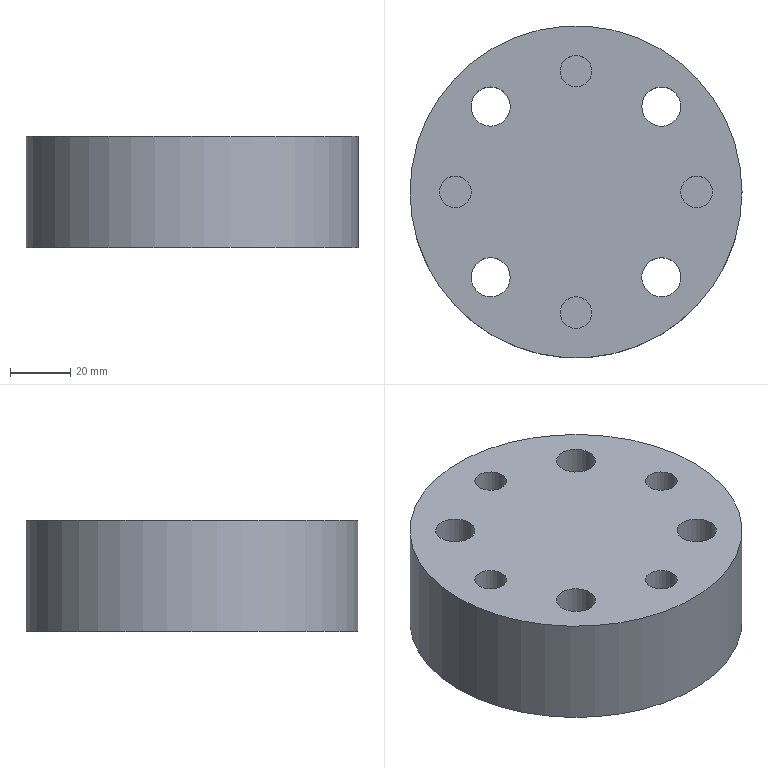NC program | NX | posted with a generic post | part box 110 x 110 x 37 mm
Whole program:
N10 G17 G21 G94 G90
(DRILLING , TOOL : ZXZ)
N12 T01 M6
N14 G54
N16 G17 G0 G90 X-28.284 Y28.284 S3000 M3
N18 G43 Z30. H1
N20 G94 G81 G98 Z-1. F250. R3.
N22 X-40. Y0.
N24 X-28.284 Y-28.284
N26 X0. Y-40.
N28 X28.284 Y-28.284
N30 X40. Y0.
N32 X28.284 Y28.284
N34 X0. Y40.
N36 G80
N38 G0 X0. Y40. Z30.
N40 M5
(DRILLING_COPY , TOOL : 13.0ZT)
N42 T03 M6
N44 G54
N46 G17 G0 G90 X28.284 Y28.284 S800 M3
N48 G43 Z30. H3
N50 G94 G73 G98 Z-41.406 F100. Q2. R3.
N52 Y-28.284
N54 X-28.284
N56 Y28.284
N58 G80
N60 G0 X-28.284 Y28.284 Z30.
N62 M5
(DRILLING_COPY_COPY , TOOL : 10.5ZT)
N64 T02 M6
N66 G54
N68 G17 G0 G90 X40. Y0. S800 M3
N70 G43 Z30. H2
N72 G94 G73 G98 Z-23.155 F100. Q2. R3.
N74 X0. Y40.
N76 X-40. Y0.
N78 X0. Y-40.
N80 G80
N82 G0 X0. Y-40. Z30.
N84 M5
(PLANAR_MILL , TOOL : D6A45)
N86 T04 M6
N88 G54
N90 G17 G0 G90 X24.114 Y-26.882 S7500 M3
N92 G43 Z30. H4
N94 Z2.
N96 G94 G1 Z-1. F1250.
N98 X23.184 Y-27.418
N100 G3 X22.684 Y-28.284 R1.
N102 X28.284 Y-33.884 R5.6
N104 X22.684 Y-28.284 R-5.6
N106 X23.184 Y-29.15 R1.
N108 G1 X24.114 Y-29.687
N110 Z2.
N112 G0 Z30.
N114 X-2.778 Y-38.515
N116 Z2.
N118 G1 Z-1.
N120 X-3.85 Y-39.134
N122 G3 X-4.35 Y-40. R1.
N124 X0. Y-44.35 R4.35
N126 X-4.35 Y-40. R-4.35
N128 X-3.85 Y-40.866 R1.
N130 G1 X-2.778 Y-41.485
N132 Z2.
N134 G0 Z30.
N136 X-32.455 Y-26.882
N138 Z2.
N140 G1 Z-1.
N142 X-33.384 Y-27.418
N144 G3 X-33.884 Y-28.284 R1.
N146 X-28.284 Y-33.884 R5.6
N148 X-33.884 Y-28.284 R-5.6
N150 X-33.384 Y-29.15 R1.
N152 G1 X-32.455 Y-29.687
N154 Z2.
N156 G0 Z30.
N158 X-42.778 Y1.485
N160 Z2.
N162 G1 Z-1.
N164 X-43.85 Y0.866
N166 G3 X-44.35 Y0. R1.
N168 X-40. Y-4.35 R4.35
N170 X-44.35 Y0. R-4.35
N172 X-43.85 Y-0.866 R1.
N174 G1 X-42.778 Y-1.485
N176 Z2.
N178 G0 Z30.
N180 X-32.455 Y29.687
N182 Z2.
N184 G1 Z-1.
N186 X-33.384 Y29.15
N188 G3 X-33.884 Y28.284 R1.
N190 X-28.284 Y22.684 R5.6
N192 X-33.884 Y28.284 R-5.6
N194 X-33.384 Y27.418 R1.
N196 G1 X-32.455 Y26.882
N198 Z2.
N200 G0 Z30.
N202 X-2.778 Y41.485
N204 Z2.
N206 G1 Z-1.
N208 X-3.85 Y40.866
N210 G3 X-4.35 Y40. R1.
N212 X0. Y35.65 R4.35
N214 X-4.35 Y40. R-4.35
N216 X-3.85 Y39.134 R1.
N218 G1 X-2.778 Y38.515
N220 Z2.
N222 G0 Z30.
N224 X24.114 Y29.687
N226 Z2.
N228 G1 Z-1.
N230 X23.184 Y29.15
N232 G3 X22.684 Y28.284 R1.
N234 X28.284 Y22.684 R5.6
N236 X22.684 Y28.284 R-5.6
N238 X23.184 Y27.418 R1.
N240 G1 X24.114 Y26.882
N242 Z2.
N244 G0 Z30.
N246 X37.222 Y1.485
N248 Z2.
N250 G1 Z-1.
N252 X36.15 Y0.866
N254 G3 X35.65 Y0. R1.
N256 X40. Y-4.35 R4.35
N258 X35.65 Y0. R-4.35
N260 X36.15 Y-0.866 R1.
N262 G1 X37.222 Y-1.485
N264 Z2.
N266 G0 Z30.
N268 M5
N270 M2